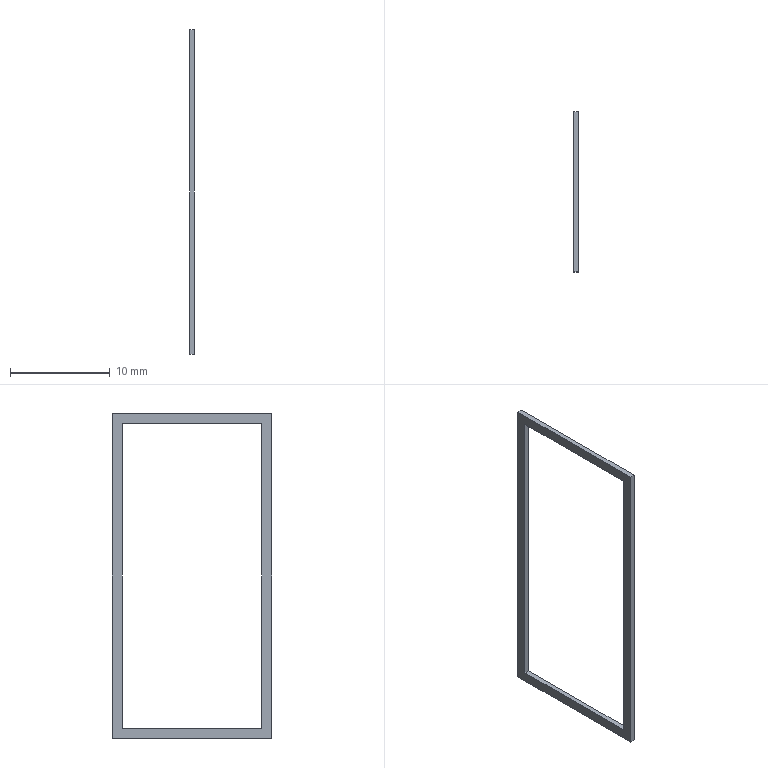Part | SolidWorks | features BaseBody 1 | 1 solid | 10 faces | box 0.5 x 16 x 32.5 mm | volume 46.5 mm3 | plane 10
STEP:
#1=CARTESIAN_POINT('',(435.1,104.75,-16.25));
#2=VERTEX_POINT('',#1);
#3=CARTESIAN_POINT('',(435.1,120.75,-16.25));
#4=VERTEX_POINT('',#3);
#5=CARTESIAN_POINT('',(435.1,104.75,-16.25));
#6=DIRECTION('',(0.,1.,0.));
#7=VECTOR('',#6,1000.);
#8=LINE('',#5,#7);
#9=EDGE_CURVE('',#2,#4,#8,.T.);
#10=ORIENTED_EDGE('',*,*,#9,.T.);
#11=CARTESIAN_POINT('',(435.1,120.75,16.25));
#12=VERTEX_POINT('',#11);
#13=CARTESIAN_POINT('',(435.1,120.75,16.25));
#14=DIRECTION('',(0.,0.,1.));
#15=VECTOR('',#14,1000.);
#16=LINE('',#13,#15);
#17=EDGE_CURVE('',#4,#12,#16,.T.);
#18=ORIENTED_EDGE('',*,*,#17,.T.);
#19=CARTESIAN_POINT('',(435.1,104.75,16.25));
#20=VERTEX_POINT('',#19);
#21=CARTESIAN_POINT('',(435.1,104.75,16.25));
#22=DIRECTION('',(0.,-1.,0.));
#23=VECTOR('',#22,1000.);
#24=LINE('',#21,#23);
#25=EDGE_CURVE('',#12,#20,#24,.T.);
#26=ORIENTED_EDGE('',*,*,#25,.T.);
#27=CARTESIAN_POINT('',(435.1,104.75,-16.25));
#28=DIRECTION('',(0.,0.,-1.));
#29=VECTOR('',#28,1000.);
#30=LINE('',#27,#29);
#31=EDGE_CURVE('',#20,#2,#30,.T.);
#32=ORIENTED_EDGE('',*,*,#31,.T.);
#33=EDGE_LOOP('',(#10,#18,#26,#32));
#34=FACE_OUTER_BOUND('',#33,.T.);
#35=CARTESIAN_POINT('',(435.1,119.75,15.25));
#36=VERTEX_POINT('',#35);
#37=CARTESIAN_POINT('',(435.1,105.75,15.25));
#38=VERTEX_POINT('',#37);
#39=CARTESIAN_POINT('',(435.1,105.75,15.25));
#40=DIRECTION('',(0.,-1.,0.));
#41=VECTOR('',#40,1000.);
#42=LINE('',#39,#41);
#43=EDGE_CURVE('',#36,#38,#42,.T.);
#44=ORIENTED_EDGE('',*,*,#43,.F.);
#45=CARTESIAN_POINT('',(435.1,119.75,-15.25));
#46=VERTEX_POINT('',#45);
#47=CARTESIAN_POINT('',(435.1,119.75,15.25));
#48=DIRECTION('',(0.,0.,1.));
#49=VECTOR('',#48,1000.);
#50=LINE('',#47,#49);
#51=EDGE_CURVE('',#46,#36,#50,.T.);
#52=ORIENTED_EDGE('',*,*,#51,.F.);
#53=CARTESIAN_POINT('',(435.1,105.75,-15.25));
#54=VERTEX_POINT('',#53);
#55=CARTESIAN_POINT('',(435.1,105.75,-15.25));
#56=DIRECTION('',(0.,1.,0.));
#57=VECTOR('',#56,1000.);
#58=LINE('',#55,#57);
#59=EDGE_CURVE('',#54,#46,#58,.T.);
#60=ORIENTED_EDGE('',*,*,#59,.F.);
#61=CARTESIAN_POINT('',(435.1,105.75,-15.25));
#62=DIRECTION('',(0.,0.,-1.));
#63=VECTOR('',#62,1000.);
#64=LINE('',#61,#63);
#65=EDGE_CURVE('',#38,#54,#64,.T.);
#66=ORIENTED_EDGE('',*,*,#65,.F.);
#67=EDGE_LOOP('',(#44,#52,#60,#66));
#68=FACE_BOUND('',#67,.T.);
#69=CARTESIAN_POINT('',(435.1,120.75,-16.25));
#70=DIRECTION('',(-1.,0.,0.));
#71=DIRECTION('',(0.,0.,1.));
#72=AXIS2_PLACEMENT_3D('',#69,#70,#71);
#73=PLANE('',#72);
#74=ADVANCED_FACE('',(#34,#68),#73,.F.);
#75=CARTESIAN_POINT('',(434.6,104.75,-16.25));
#76=VERTEX_POINT('',#75);
#77=CARTESIAN_POINT('',(434.6,120.75,-16.25));
#78=VERTEX_POINT('',#77);
#79=CARTESIAN_POINT('',(434.6,104.75,-16.25));
#80=DIRECTION('',(0.,1.,0.));
#81=VECTOR('',#80,1000.);
#82=LINE('',#79,#81);
#83=EDGE_CURVE('',#76,#78,#82,.T.);
#84=ORIENTED_EDGE('',*,*,#83,.F.);
#85=CARTESIAN_POINT('',(434.6,104.75,16.25));
#86=VERTEX_POINT('',#85);
#87=CARTESIAN_POINT('',(434.6,104.75,-16.25));
#88=DIRECTION('',(0.,0.,-1.));
#89=VECTOR('',#88,1000.);
#90=LINE('',#87,#89);
#91=EDGE_CURVE('',#86,#76,#90,.T.);
#92=ORIENTED_EDGE('',*,*,#91,.F.);
#93=CARTESIAN_POINT('',(434.6,120.75,16.25));
#94=VERTEX_POINT('',#93);
#95=CARTESIAN_POINT('',(434.6,104.75,16.25));
#96=DIRECTION('',(0.,-1.,0.));
#97=VECTOR('',#96,1000.);
#98=LINE('',#95,#97);
#99=EDGE_CURVE('',#94,#86,#98,.T.);
#100=ORIENTED_EDGE('',*,*,#99,.F.);
#101=CARTESIAN_POINT('',(434.6,120.75,16.25));
#102=DIRECTION('',(0.,0.,1.));
#103=VECTOR('',#102,1000.);
#104=LINE('',#101,#103);
#105=EDGE_CURVE('',#78,#94,#104,.T.);
#106=ORIENTED_EDGE('',*,*,#105,.F.);
#107=EDGE_LOOP('',(#84,#92,#100,#106));
#108=FACE_OUTER_BOUND('',#107,.T.);
#109=CARTESIAN_POINT('',(434.6,119.75,-15.25));
#110=VERTEX_POINT('',#109);
#111=CARTESIAN_POINT('',(434.6,119.75,15.25));
#112=VERTEX_POINT('',#111);
#113=CARTESIAN_POINT('',(434.6,119.75,15.25));
#114=DIRECTION('',(0.,0.,1.));
#115=VECTOR('',#114,1000.);
#116=LINE('',#113,#115);
#117=EDGE_CURVE('',#110,#112,#116,.T.);
#118=ORIENTED_EDGE('',*,*,#117,.T.);
#119=CARTESIAN_POINT('',(434.6,105.75,15.25));
#120=VERTEX_POINT('',#119);
#121=CARTESIAN_POINT('',(434.6,105.75,15.25));
#122=DIRECTION('',(0.,-1.,0.));
#123=VECTOR('',#122,1000.);
#124=LINE('',#121,#123);
#125=EDGE_CURVE('',#112,#120,#124,.T.);
#126=ORIENTED_EDGE('',*,*,#125,.T.);
#127=CARTESIAN_POINT('',(434.6,105.75,-15.25));
#128=VERTEX_POINT('',#127);
#129=CARTESIAN_POINT('',(434.6,105.75,-15.25));
#130=DIRECTION('',(0.,0.,-1.));
#131=VECTOR('',#130,1000.);
#132=LINE('',#129,#131);
#133=EDGE_CURVE('',#120,#128,#132,.T.);
#134=ORIENTED_EDGE('',*,*,#133,.T.);
#135=CARTESIAN_POINT('',(434.6,105.75,-15.25));
#136=DIRECTION('',(0.,1.,0.));
#137=VECTOR('',#136,1000.);
#138=LINE('',#135,#137);
#139=EDGE_CURVE('',#128,#110,#138,.T.);
#140=ORIENTED_EDGE('',*,*,#139,.T.);
#141=EDGE_LOOP('',(#118,#126,#134,#140));
#142=FACE_BOUND('',#141,.T.);
#143=CARTESIAN_POINT('',(434.6,120.75,-16.25));
#144=DIRECTION('',(-1.,0.,0.));
#145=DIRECTION('',(0.,0.,1.));
#146=AXIS2_PLACEMENT_3D('',#143,#144,#145);
#147=PLANE('',#146);
#148=ADVANCED_FACE('',(#108,#142),#147,.T.);
#149=ORIENTED_EDGE('',*,*,#83,.T.);
#150=CARTESIAN_POINT('',(435.1,120.75,-16.25));
#151=DIRECTION('',(-1.,0.,0.));
#152=VECTOR('',#151,1000.);
#153=LINE('',#150,#152);
#154=EDGE_CURVE('',#4,#78,#153,.T.);
#155=ORIENTED_EDGE('',*,*,#154,.F.);
#156=ORIENTED_EDGE('',*,*,#9,.F.);
#157=CARTESIAN_POINT('',(435.1,104.75,-16.25));
#158=DIRECTION('',(-1.,0.,0.));
#159=VECTOR('',#158,1000.);
#160=LINE('',#157,#159);
#161=EDGE_CURVE('',#2,#76,#160,.T.);
#162=ORIENTED_EDGE('',*,*,#161,.T.);
#163=EDGE_LOOP('',(#149,#155,#156,#162));
#164=FACE_OUTER_BOUND('',#163,.T.);
#165=CARTESIAN_POINT('',(435.1,104.75,-16.25));
#166=DIRECTION('',(0.,0.,1.));
#167=DIRECTION('',(1.,0.,0.));
#168=AXIS2_PLACEMENT_3D('',#165,#166,#167);
#169=PLANE('',#168);
#170=ADVANCED_FACE('',(#164),#169,.F.);
#171=ORIENTED_EDGE('',*,*,#105,.T.);
#172=CARTESIAN_POINT('',(435.1,120.75,16.25));
#173=DIRECTION('',(-1.,0.,0.));
#174=VECTOR('',#173,1000.);
#175=LINE('',#172,#174);
#176=EDGE_CURVE('',#12,#94,#175,.T.);
#177=ORIENTED_EDGE('',*,*,#176,.F.);
#178=ORIENTED_EDGE('',*,*,#17,.F.);
#179=ORIENTED_EDGE('',*,*,#154,.T.);
#180=EDGE_LOOP('',(#171,#177,#178,#179));
#181=FACE_OUTER_BOUND('',#180,.T.);
#182=CARTESIAN_POINT('',(435.1,120.75,16.25));
#183=DIRECTION('',(0.,-1.,0.));
#184=DIRECTION('',(-1.,0.,0.));
#185=AXIS2_PLACEMENT_3D('',#182,#183,#184);
#186=PLANE('',#185);
#187=ADVANCED_FACE('',(#181),#186,.F.);
#188=ORIENTED_EDGE('',*,*,#99,.T.);
#189=CARTESIAN_POINT('',(435.1,104.75,16.25));
#190=DIRECTION('',(-1.,0.,0.));
#191=VECTOR('',#190,1000.);
#192=LINE('',#189,#191);
#193=EDGE_CURVE('',#20,#86,#192,.T.);
#194=ORIENTED_EDGE('',*,*,#193,.F.);
#195=ORIENTED_EDGE('',*,*,#25,.F.);
#196=ORIENTED_EDGE('',*,*,#176,.T.);
#197=EDGE_LOOP('',(#188,#194,#195,#196));
#198=FACE_OUTER_BOUND('',#197,.T.);
#199=CARTESIAN_POINT('',(435.1,104.75,16.25));
#200=DIRECTION('',(0.,0.,-1.));
#201=DIRECTION('',(-1.,0.,0.));
#202=AXIS2_PLACEMENT_3D('',#199,#200,#201);
#203=PLANE('',#202);
#204=ADVANCED_FACE('',(#198),#203,.F.);
#205=ORIENTED_EDGE('',*,*,#91,.T.);
#206=ORIENTED_EDGE('',*,*,#161,.F.);
#207=ORIENTED_EDGE('',*,*,#31,.F.);
#208=ORIENTED_EDGE('',*,*,#193,.T.);
#209=EDGE_LOOP('',(#205,#206,#207,#208));
#210=FACE_OUTER_BOUND('',#209,.T.);
#211=CARTESIAN_POINT('',(435.1,104.75,-16.25));
#212=DIRECTION('',(0.,1.,0.));
#213=DIRECTION('',(0.,0.,1.));
#214=AXIS2_PLACEMENT_3D('',#211,#212,#213);
#215=PLANE('',#214);
#216=ADVANCED_FACE('',(#210),#215,.F.);
#217=ORIENTED_EDGE('',*,*,#125,.F.);
#218=CARTESIAN_POINT('',(435.1,119.75,15.25));
#219=DIRECTION('',(-1.,0.,0.));
#220=VECTOR('',#219,1000.);
#221=LINE('',#218,#220);
#222=EDGE_CURVE('',#36,#112,#221,.T.);
#223=ORIENTED_EDGE('',*,*,#222,.F.);
#224=ORIENTED_EDGE('',*,*,#43,.T.);
#225=CARTESIAN_POINT('',(435.1,105.75,15.25));
#226=DIRECTION('',(-1.,0.,0.));
#227=VECTOR('',#226,1000.);
#228=LINE('',#225,#227);
#229=EDGE_CURVE('',#38,#120,#228,.T.);
#230=ORIENTED_EDGE('',*,*,#229,.T.);
#231=EDGE_LOOP('',(#217,#223,#224,#230));
#232=FACE_OUTER_BOUND('',#231,.T.);
#233=CARTESIAN_POINT('',(435.1,105.75,15.25));
#234=DIRECTION('',(0.,0.,-1.));
#235=DIRECTION('',(-1.,0.,0.));
#236=AXIS2_PLACEMENT_3D('',#233,#234,#235);
#237=PLANE('',#236);
#238=ADVANCED_FACE('',(#232),#237,.T.);
#239=ORIENTED_EDGE('',*,*,#133,.F.);
#240=ORIENTED_EDGE('',*,*,#229,.F.);
#241=ORIENTED_EDGE('',*,*,#65,.T.);
#242=CARTESIAN_POINT('',(435.1,105.75,-15.25));
#243=DIRECTION('',(-1.,0.,0.));
#244=VECTOR('',#243,1000.);
#245=LINE('',#242,#244);
#246=EDGE_CURVE('',#54,#128,#245,.T.);
#247=ORIENTED_EDGE('',*,*,#246,.T.);
#248=EDGE_LOOP('',(#239,#240,#241,#247));
#249=FACE_OUTER_BOUND('',#248,.T.);
#250=CARTESIAN_POINT('',(435.1,105.75,-15.25));
#251=DIRECTION('',(0.,1.,0.));
#252=DIRECTION('',(0.,0.,1.));
#253=AXIS2_PLACEMENT_3D('',#250,#251,#252);
#254=PLANE('',#253);
#255=ADVANCED_FACE('',(#249),#254,.T.);
#256=ORIENTED_EDGE('',*,*,#139,.F.);
#257=ORIENTED_EDGE('',*,*,#246,.F.);
#258=ORIENTED_EDGE('',*,*,#59,.T.);
#259=CARTESIAN_POINT('',(435.1,119.75,-15.25));
#260=DIRECTION('',(-1.,0.,0.));
#261=VECTOR('',#260,1000.);
#262=LINE('',#259,#261);
#263=EDGE_CURVE('',#46,#110,#262,.T.);
#264=ORIENTED_EDGE('',*,*,#263,.T.);
#265=EDGE_LOOP('',(#256,#257,#258,#264));
#266=FACE_OUTER_BOUND('',#265,.T.);
#267=CARTESIAN_POINT('',(435.1,105.75,-15.25));
#268=DIRECTION('',(0.,0.,1.));
#269=DIRECTION('',(1.,0.,0.));
#270=AXIS2_PLACEMENT_3D('',#267,#268,#269);
#271=PLANE('',#270);
#272=ADVANCED_FACE('',(#266),#271,.T.);
#273=ORIENTED_EDGE('',*,*,#117,.F.);
#274=ORIENTED_EDGE('',*,*,#263,.F.);
#275=ORIENTED_EDGE('',*,*,#51,.T.);
#276=ORIENTED_EDGE('',*,*,#222,.T.);
#277=EDGE_LOOP('',(#273,#274,#275,#276));
#278=FACE_OUTER_BOUND('',#277,.T.);
#279=CARTESIAN_POINT('',(435.1,119.75,15.25));
#280=DIRECTION('',(0.,-1.,0.));
#281=DIRECTION('',(-1.,0.,0.));
#282=AXIS2_PLACEMENT_3D('',#279,#280,#281);
#283=PLANE('',#282);
#284=ADVANCED_FACE('',(#278),#283,.T.);
#285=CLOSED_SHELL('',(#74,#148,#170,#187,#204,#216,#238,#255,#272,#284));
#286=MANIFOLD_SOLID_BREP('',#285);
#287=CARTESIAN_POINT('',(0.,0.,0.));
#288=DIRECTION('',(0.,0.,1.));
#289=DIRECTION('',(1.,0.,0.));
#290=AXIS2_PLACEMENT_3D('',#287,#288,#289);
#291=(LENGTH_UNIT()NAMED_UNIT(*)SI_UNIT(.MILLI.,.METRE.));
#292=UNCERTAINTY_MEASURE_WITH_UNIT(LENGTH_MEASURE(0.00001),#291,'','');
#293=(NAMED_UNIT(*)PLANE_ANGLE_UNIT()SI_UNIT($,.RADIAN.));
#294=(NAMED_UNIT(*)SI_UNIT($,.STERADIAN.)SOLID_ANGLE_UNIT());
#295=(GEOMETRIC_REPRESENTATION_CONTEXT(3)GLOBAL_UNCERTAINTY_ASSIGNED_CONTEXT((#292))GLOBAL_UNIT_ASSIGNED_CONTEXT((#291,#293,#294))REPRESENTATION_CONTEXT('',''));
#296=ADVANCED_BREP_SHAPE_REPRESENTATION('',(#286,#290),#295);